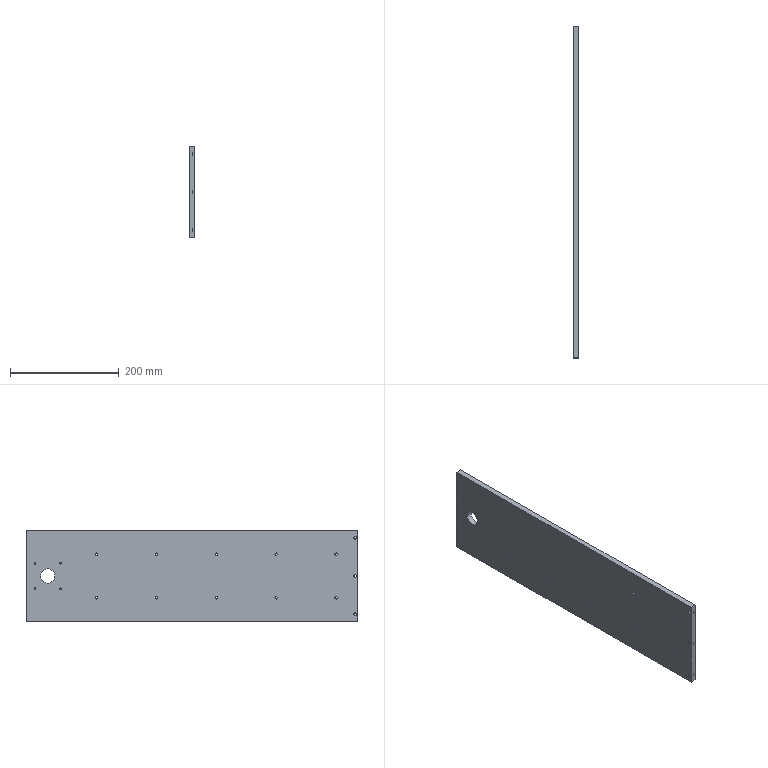Part | STEP file | 03-07 Feed mechanism support plate | 1 solid | 93 faces | box 10 x 609 x 168 mm | volume 1012240 mm3 | cylinder 68 | plane 19 | cone 6 | commonest cylinder face diameters 4.5 x26 9 x26 3.3 x14 26 x2